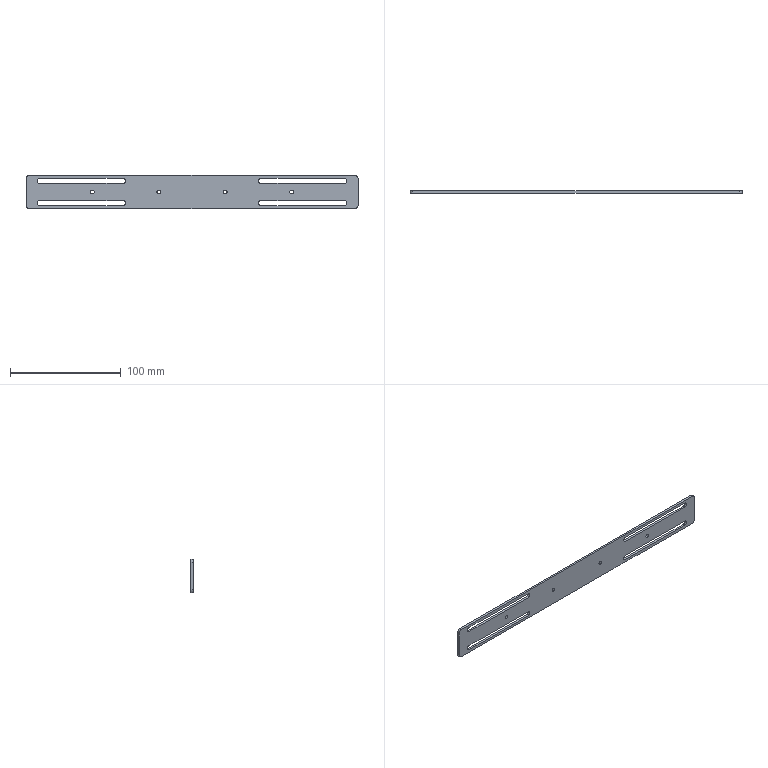Part | SolidWorks | features HoleWzd 2, Fillet 1, FlatPattern 1, SMBaseFlange 1, SheetMetal 1 | 1 solid | 34 faces | box 300 x 2 x 30 mm | volume 15076 mm3 | cylinder 20 | plane 14 | commonest cylinder face diameters 3.3 x8 4.5 x8 5 x4
STEP:
#1=CARTESIAN_POINT('',(-30.,-2.,-1.65));
#2=VERTEX_POINT('',#1);
#3=CARTESIAN_POINT('',(-30.,-2.,1.65));
#4=VERTEX_POINT('',#3);
#5=CARTESIAN_POINT('',(-30.,-2.,0.));
#6=DIRECTION('',(0.,1.,0.));
#7=DIRECTION('',(0.,0.,1.));
#8=AXIS2_PLACEMENT_3D('',#5,#6,#7);
#9=CIRCLE('',#8,1.65);
#10=EDGE_CURVE('',#2,#4,#9,.T.);
#11=ORIENTED_EDGE('',*,*,#10,.F.);
#12=CARTESIAN_POINT('',(-30.,0.,-1.65));
#13=VERTEX_POINT('',#12);
#14=CARTESIAN_POINT('',(-30.,0.,-1.65));
#15=DIRECTION('',(0.,1.,0.));
#16=VECTOR('',#15,1000.);
#17=LINE('',#14,#16);
#18=EDGE_CURVE('',#2,#13,#17,.T.);
#19=ORIENTED_EDGE('',*,*,#18,.T.);
#20=CARTESIAN_POINT('',(-30.,0.,1.65));
#21=VERTEX_POINT('',#20);
#22=CARTESIAN_POINT('',(-30.,0.,0.));
#23=DIRECTION('',(0.,1.,0.));
#24=DIRECTION('',(0.,0.,1.));
#25=AXIS2_PLACEMENT_3D('',#22,#23,#24);
#26=CIRCLE('',#25,1.65);
#27=EDGE_CURVE('',#13,#21,#26,.T.);
#28=ORIENTED_EDGE('',*,*,#27,.T.);
#29=CARTESIAN_POINT('',(-30.,0.,1.65));
#30=DIRECTION('',(0.,1.,0.));
#31=VECTOR('',#30,1000.);
#32=LINE('',#29,#31);
#33=EDGE_CURVE('',#4,#21,#32,.T.);
#34=ORIENTED_EDGE('',*,*,#33,.F.);
#35=EDGE_LOOP('',(#11,#19,#28,#34));
#36=FACE_OUTER_BOUND('',#35,.T.);
#37=CARTESIAN_POINT('',(-30.,0.,0.));
#38=DIRECTION('',(0.,1.,0.));
#39=DIRECTION('',(0.,0.,1.));
#40=AXIS2_PLACEMENT_3D('',#37,#38,#39);
#41=CYLINDRICAL_SURFACE('',#40,1.65);
#42=ADVANCED_FACE('',(#36),#41,.F.);
#43=CARTESIAN_POINT('',(30.,-2.,-1.65));
#44=VERTEX_POINT('',#43);
#45=CARTESIAN_POINT('',(30.,-2.,1.65));
#46=VERTEX_POINT('',#45);
#47=CARTESIAN_POINT('',(30.,-2.,0.));
#48=DIRECTION('',(0.,1.,0.));
#49=DIRECTION('',(0.,0.,1.));
#50=AXIS2_PLACEMENT_3D('',#47,#48,#49);
#51=CIRCLE('',#50,1.65);
#52=EDGE_CURVE('',#44,#46,#51,.T.);
#53=ORIENTED_EDGE('',*,*,#52,.F.);
#54=CARTESIAN_POINT('',(30.,0.,-1.65));
#55=VERTEX_POINT('',#54);
#56=CARTESIAN_POINT('',(30.,0.,-1.65));
#57=DIRECTION('',(0.,1.,0.));
#58=VECTOR('',#57,1000.);
#59=LINE('',#56,#58);
#60=EDGE_CURVE('',#44,#55,#59,.T.);
#61=ORIENTED_EDGE('',*,*,#60,.T.);
#62=CARTESIAN_POINT('',(30.,0.,1.65));
#63=VERTEX_POINT('',#62);
#64=CARTESIAN_POINT('',(30.,0.,0.));
#65=DIRECTION('',(0.,1.,0.));
#66=DIRECTION('',(0.,0.,1.));
#67=AXIS2_PLACEMENT_3D('',#64,#65,#66);
#68=CIRCLE('',#67,1.65);
#69=EDGE_CURVE('',#55,#63,#68,.T.);
#70=ORIENTED_EDGE('',*,*,#69,.T.);
#71=CARTESIAN_POINT('',(30.,0.,1.65));
#72=DIRECTION('',(0.,1.,0.));
#73=VECTOR('',#72,1000.);
#74=LINE('',#71,#73);
#75=EDGE_CURVE('',#46,#63,#74,.T.);
#76=ORIENTED_EDGE('',*,*,#75,.F.);
#77=EDGE_LOOP('',(#53,#61,#70,#76));
#78=FACE_OUTER_BOUND('',#77,.T.);
#79=CARTESIAN_POINT('',(30.,0.,0.));
#80=DIRECTION('',(0.,1.,0.));
#81=DIRECTION('',(0.,0.,1.));
#82=AXIS2_PLACEMENT_3D('',#79,#80,#81);
#83=CYLINDRICAL_SURFACE('',#82,1.65);
#84=ADVANCED_FACE('',(#78),#83,.F.);
#85=CARTESIAN_POINT('',(-90.,-2.,-1.65));
#86=VERTEX_POINT('',#85);
#87=CARTESIAN_POINT('',(-90.,-2.,1.65));
#88=VERTEX_POINT('',#87);
#89=CARTESIAN_POINT('',(-90.,-2.,0.));
#90=DIRECTION('',(0.,1.,0.));
#91=DIRECTION('',(0.,0.,1.));
#92=AXIS2_PLACEMENT_3D('',#89,#90,#91);
#93=CIRCLE('',#92,1.65);
#94=EDGE_CURVE('',#86,#88,#93,.T.);
#95=ORIENTED_EDGE('',*,*,#94,.F.);
#96=CARTESIAN_POINT('',(-90.,0.,-1.65));
#97=VERTEX_POINT('',#96);
#98=CARTESIAN_POINT('',(-90.,0.,-1.65));
#99=DIRECTION('',(0.,1.,0.));
#100=VECTOR('',#99,1000.);
#101=LINE('',#98,#100);
#102=EDGE_CURVE('',#86,#97,#101,.T.);
#103=ORIENTED_EDGE('',*,*,#102,.T.);
#104=CARTESIAN_POINT('',(-90.,0.,1.65));
#105=VERTEX_POINT('',#104);
#106=CARTESIAN_POINT('',(-90.,0.,0.));
#107=DIRECTION('',(0.,1.,0.));
#108=DIRECTION('',(0.,0.,1.));
#109=AXIS2_PLACEMENT_3D('',#106,#107,#108);
#110=CIRCLE('',#109,1.65);
#111=EDGE_CURVE('',#97,#105,#110,.T.);
#112=ORIENTED_EDGE('',*,*,#111,.T.);
#113=CARTESIAN_POINT('',(-90.,0.,1.65));
#114=DIRECTION('',(0.,1.,0.));
#115=VECTOR('',#114,1000.);
#116=LINE('',#113,#115);
#117=EDGE_CURVE('',#88,#105,#116,.T.);
#118=ORIENTED_EDGE('',*,*,#117,.F.);
#119=EDGE_LOOP('',(#95,#103,#112,#118));
#120=FACE_OUTER_BOUND('',#119,.T.);
#121=CARTESIAN_POINT('',(-90.,0.,0.));
#122=DIRECTION('',(0.,1.,0.));
#123=DIRECTION('',(0.,0.,1.));
#124=AXIS2_PLACEMENT_3D('',#121,#122,#123);
#125=CYLINDRICAL_SURFACE('',#124,1.65);
#126=ADVANCED_FACE('',(#120),#125,.F.);
#127=CARTESIAN_POINT('',(90.,-2.,-1.65));
#128=VERTEX_POINT('',#127);
#129=CARTESIAN_POINT('',(90.,-2.,1.65));
#130=VERTEX_POINT('',#129);
#131=CARTESIAN_POINT('',(90.,-2.,0.));
#132=DIRECTION('',(0.,1.,0.));
#133=DIRECTION('',(0.,0.,1.));
#134=AXIS2_PLACEMENT_3D('',#131,#132,#133);
#135=CIRCLE('',#134,1.65);
#136=EDGE_CURVE('',#128,#130,#135,.T.);
#137=ORIENTED_EDGE('',*,*,#136,.F.);
#138=CARTESIAN_POINT('',(90.,0.,-1.65));
#139=VERTEX_POINT('',#138);
#140=CARTESIAN_POINT('',(90.,0.,-1.65));
#141=DIRECTION('',(0.,1.,0.));
#142=VECTOR('',#141,1000.);
#143=LINE('',#140,#142);
#144=EDGE_CURVE('',#128,#139,#143,.T.);
#145=ORIENTED_EDGE('',*,*,#144,.T.);
#146=CARTESIAN_POINT('',(90.,0.,1.65));
#147=VERTEX_POINT('',#146);
#148=CARTESIAN_POINT('',(90.,0.,0.));
#149=DIRECTION('',(0.,1.,0.));
#150=DIRECTION('',(0.,0.,1.));
#151=AXIS2_PLACEMENT_3D('',#148,#149,#150);
#152=CIRCLE('',#151,1.65);
#153=EDGE_CURVE('',#139,#147,#152,.T.);
#154=ORIENTED_EDGE('',*,*,#153,.T.);
#155=CARTESIAN_POINT('',(90.,0.,1.65));
#156=DIRECTION('',(0.,1.,0.));
#157=VECTOR('',#156,1000.);
#158=LINE('',#155,#157);
#159=EDGE_CURVE('',#130,#147,#158,.T.);
#160=ORIENTED_EDGE('',*,*,#159,.F.);
#161=EDGE_LOOP('',(#137,#145,#154,#160));
#162=FACE_OUTER_BOUND('',#161,.T.);
#163=CARTESIAN_POINT('',(90.,0.,0.));
#164=DIRECTION('',(0.,1.,0.));
#165=DIRECTION('',(0.,0.,1.));
#166=AXIS2_PLACEMENT_3D('',#163,#164,#165);
#167=CYLINDRICAL_SURFACE('',#166,1.65);
#168=ADVANCED_FACE('',(#162),#167,.F.);
#169=CARTESIAN_POINT('',(147.5,-2.,-15.));
#170=VERTEX_POINT('',#169);
#171=CARTESIAN_POINT('',(-147.5,-2.,-15.));
#172=VERTEX_POINT('',#171);
#173=CARTESIAN_POINT('',(-150.,-2.,-15.));
#174=DIRECTION('',(-1.,0.,0.));
#175=VECTOR('',#174,1000.);
#176=LINE('',#173,#175);
#177=EDGE_CURVE('',#170,#172,#176,.T.);
#178=ORIENTED_EDGE('',*,*,#177,.F.);
#179=CARTESIAN_POINT('',(150.,-2.,-12.5));
#180=VERTEX_POINT('',#179);
#181=CARTESIAN_POINT('',(147.5,-2.,-12.5));
#182=DIRECTION('',(0.,-1.,0.));
#183=DIRECTION('',(0.,0.,1.));
#184=AXIS2_PLACEMENT_3D('',#181,#182,#183);
#185=CIRCLE('',#184,2.5);
#186=EDGE_CURVE('',#170,#180,#185,.T.);
#187=ORIENTED_EDGE('',*,*,#186,.T.);
#188=CARTESIAN_POINT('',(150.,-2.,12.5));
#189=VERTEX_POINT('',#188);
#190=CARTESIAN_POINT('',(150.,-2.,-15.));
#191=DIRECTION('',(0.,0.,-1.));
#192=VECTOR('',#191,1000.);
#193=LINE('',#190,#192);
#194=EDGE_CURVE('',#189,#180,#193,.T.);
#195=ORIENTED_EDGE('',*,*,#194,.F.);
#196=CARTESIAN_POINT('',(147.5,-2.,15.));
#197=VERTEX_POINT('',#196);
#198=CARTESIAN_POINT('',(147.5,-2.,12.5));
#199=DIRECTION('',(0.,-1.,0.));
#200=DIRECTION('',(0.,0.,1.));
#201=AXIS2_PLACEMENT_3D('',#198,#199,#200);
#202=CIRCLE('',#201,2.5);
#203=EDGE_CURVE('',#189,#197,#202,.T.);
#204=ORIENTED_EDGE('',*,*,#203,.T.);
#205=CARTESIAN_POINT('',(-147.5,-2.,15.));
#206=VERTEX_POINT('',#205);
#207=CARTESIAN_POINT('',(-150.,-2.,15.));
#208=DIRECTION('',(1.,0.,0.));
#209=VECTOR('',#208,1000.);
#210=LINE('',#207,#209);
#211=EDGE_CURVE('',#206,#197,#210,.T.);
#212=ORIENTED_EDGE('',*,*,#211,.F.);
#213=CARTESIAN_POINT('',(-150.,-2.,12.5));
#214=VERTEX_POINT('',#213);
#215=CARTESIAN_POINT('',(-147.5,-2.,12.5));
#216=DIRECTION('',(0.,-1.,0.));
#217=DIRECTION('',(0.,0.,1.));
#218=AXIS2_PLACEMENT_3D('',#215,#216,#217);
#219=CIRCLE('',#218,2.5);
#220=EDGE_CURVE('',#206,#214,#219,.T.);
#221=ORIENTED_EDGE('',*,*,#220,.T.);
#222=CARTESIAN_POINT('',(-150.,-2.,-12.5));
#223=VERTEX_POINT('',#222);
#224=CARTESIAN_POINT('',(-150.,-2.,-15.));
#225=DIRECTION('',(0.,0.,1.));
#226=VECTOR('',#225,1000.);
#227=LINE('',#224,#226);
#228=EDGE_CURVE('',#223,#214,#227,.T.);
#229=ORIENTED_EDGE('',*,*,#228,.F.);
#230=CARTESIAN_POINT('',(-147.5,-2.,-12.5));
#231=DIRECTION('',(0.,-1.,0.));
#232=DIRECTION('',(0.,0.,1.));
#233=AXIS2_PLACEMENT_3D('',#230,#231,#232);
#234=CIRCLE('',#233,2.5);
#235=EDGE_CURVE('',#223,#172,#234,.T.);
#236=ORIENTED_EDGE('',*,*,#235,.T.);
#237=EDGE_LOOP('',(#178,#187,#195,#204,#212,#221,#229,#236));
#238=FACE_OUTER_BOUND('',#237,.T.);
#239=CARTESIAN_POINT('',(90.,-2.,0.));
#240=DIRECTION('',(0.,1.,0.));
#241=DIRECTION('',(0.,0.,1.));
#242=AXIS2_PLACEMENT_3D('',#239,#240,#241);
#243=CIRCLE('',#242,1.65);
#244=EDGE_CURVE('',#130,#128,#243,.T.);
#245=ORIENTED_EDGE('',*,*,#244,.T.);
#246=ORIENTED_EDGE('',*,*,#136,.T.);
#247=EDGE_LOOP('',(#245,#246));
#248=FACE_BOUND('',#247,.T.);
#249=CARTESIAN_POINT('',(-90.,-2.,0.));
#250=DIRECTION('',(0.,1.,0.));
#251=DIRECTION('',(0.,0.,1.));
#252=AXIS2_PLACEMENT_3D('',#249,#250,#251);
#253=CIRCLE('',#252,1.65);
#254=EDGE_CURVE('',#88,#86,#253,.T.);
#255=ORIENTED_EDGE('',*,*,#254,.T.);
#256=ORIENTED_EDGE('',*,*,#94,.T.);
#257=EDGE_LOOP('',(#255,#256));
#258=FACE_BOUND('',#257,.T.);
#259=CARTESIAN_POINT('',(30.,-2.,0.));
#260=DIRECTION('',(0.,1.,0.));
#261=DIRECTION('',(0.,0.,1.));
#262=AXIS2_PLACEMENT_3D('',#259,#260,#261);
#263=CIRCLE('',#262,1.65);
#264=EDGE_CURVE('',#46,#44,#263,.T.);
#265=ORIENTED_EDGE('',*,*,#264,.T.);
#266=ORIENTED_EDGE('',*,*,#52,.T.);
#267=EDGE_LOOP('',(#265,#266));
#268=FACE_BOUND('',#267,.T.);
#269=CARTESIAN_POINT('',(-30.,-2.,0.));
#270=DIRECTION('',(0.,1.,0.));
#271=DIRECTION('',(0.,0.,1.));
#272=AXIS2_PLACEMENT_3D('',#269,#270,#271);
#273=CIRCLE('',#272,1.65);
#274=EDGE_CURVE('',#4,#2,#273,.T.);
#275=ORIENTED_EDGE('',*,*,#274,.T.);
#276=ORIENTED_EDGE('',*,*,#10,.T.);
#277=EDGE_LOOP('',(#275,#276));
#278=FACE_BOUND('',#277,.T.);
#279=CARTESIAN_POINT('',(-62.25,-2.,-12.25));
#280=VERTEX_POINT('',#279);
#281=CARTESIAN_POINT('',(-62.25,-2.,-7.75));
#282=VERTEX_POINT('',#281);
#283=CARTESIAN_POINT('',(-62.25,-2.,-10.));
#284=DIRECTION('',(0.,-1.,0.));
#285=DIRECTION('',(0.,0.,-1.));
#286=AXIS2_PLACEMENT_3D('',#283,#284,#285);
#287=CIRCLE('',#286,2.25);
#288=EDGE_CURVE('',#280,#282,#287,.T.);
#289=ORIENTED_EDGE('',*,*,#288,.F.);
#290=CARTESIAN_POINT('',(-137.75,-2.,-12.25));
#291=VERTEX_POINT('',#290);
#292=CARTESIAN_POINT('',(-137.75,-2.,-12.25));
#293=DIRECTION('',(1.,0.,0.));
#294=VECTOR('',#293,1000.);
#295=LINE('',#292,#294);
#296=EDGE_CURVE('',#291,#280,#295,.T.);
#297=ORIENTED_EDGE('',*,*,#296,.F.);
#298=CARTESIAN_POINT('',(-137.75,-2.,-7.75));
#299=VERTEX_POINT('',#298);
#300=CARTESIAN_POINT('',(-137.75,-2.,-10.));
#301=DIRECTION('',(0.,-1.,0.));
#302=DIRECTION('',(0.,0.,-1.));
#303=AXIS2_PLACEMENT_3D('',#300,#301,#302);
#304=CIRCLE('',#303,2.25);
#305=EDGE_CURVE('',#299,#291,#304,.T.);
#306=ORIENTED_EDGE('',*,*,#305,.F.);
#307=CARTESIAN_POINT('',(-137.75,-2.,-7.75));
#308=DIRECTION('',(1.,0.,0.));
#309=VECTOR('',#308,1000.);
#310=LINE('',#307,#309);
#311=EDGE_CURVE('',#299,#282,#310,.T.);
#312=ORIENTED_EDGE('',*,*,#311,.T.);
#313=EDGE_LOOP('',(#289,#297,#306,#312));
#314=FACE_BOUND('',#313,.T.);
#315=CARTESIAN_POINT('',(62.25,-2.,-7.75));
#316=VERTEX_POINT('',#315);
#317=CARTESIAN_POINT('',(137.75,-2.,-7.75));
#318=VERTEX_POINT('',#317);
#319=CARTESIAN_POINT('',(62.25,-2.,-7.75));
#320=DIRECTION('',(1.,0.,0.));
#321=VECTOR('',#320,1000.);
#322=LINE('',#319,#321);
#323=EDGE_CURVE('',#316,#318,#322,.T.);
#324=ORIENTED_EDGE('',*,*,#323,.T.);
#325=CARTESIAN_POINT('',(137.75,-2.,-12.25));
#326=VERTEX_POINT('',#325);
#327=CARTESIAN_POINT('',(137.75,-2.,-10.));
#328=DIRECTION('',(0.,-1.,0.));
#329=DIRECTION('',(0.,0.,-1.));
#330=AXIS2_PLACEMENT_3D('',#327,#328,#329);
#331=CIRCLE('',#330,2.25);
#332=EDGE_CURVE('',#326,#318,#331,.T.);
#333=ORIENTED_EDGE('',*,*,#332,.F.);
#334=CARTESIAN_POINT('',(62.25,-2.,-12.25));
#335=VERTEX_POINT('',#334);
#336=CARTESIAN_POINT('',(62.25,-2.,-12.25));
#337=DIRECTION('',(1.,0.,0.));
#338=VECTOR('',#337,1000.);
#339=LINE('',#336,#338);
#340=EDGE_CURVE('',#335,#326,#339,.T.);
#341=ORIENTED_EDGE('',*,*,#340,.F.);
#342=CARTESIAN_POINT('',(62.25,-2.,-10.));
#343=DIRECTION('',(0.,-1.,0.));
#344=DIRECTION('',(0.,0.,-1.));
#345=AXIS2_PLACEMENT_3D('',#342,#343,#344);
#346=CIRCLE('',#345,2.25);
#347=EDGE_CURVE('',#316,#335,#346,.T.);
#348=ORIENTED_EDGE('',*,*,#347,.F.);
#349=EDGE_LOOP('',(#324,#333,#341,#348));
#350=FACE_BOUND('',#349,.T.);
#351=CARTESIAN_POINT('',(62.25,-2.,12.25));
#352=VERTEX_POINT('',#351);
#353=CARTESIAN_POINT('',(62.25,-2.,7.75));
#354=VERTEX_POINT('',#353);
#355=CARTESIAN_POINT('',(62.25,-2.,10.));
#356=DIRECTION('',(0.,-1.,0.));
#357=DIRECTION('',(0.,0.,-1.));
#358=AXIS2_PLACEMENT_3D('',#355,#356,#357);
#359=CIRCLE('',#358,2.25);
#360=EDGE_CURVE('',#352,#354,#359,.T.);
#361=ORIENTED_EDGE('',*,*,#360,.F.);
#362=CARTESIAN_POINT('',(137.75,-2.,12.25));
#363=VERTEX_POINT('',#362);
#364=CARTESIAN_POINT('',(62.25,-2.,12.25));
#365=DIRECTION('',(1.,0.,0.));
#366=VECTOR('',#365,1000.);
#367=LINE('',#364,#366);
#368=EDGE_CURVE('',#352,#363,#367,.T.);
#369=ORIENTED_EDGE('',*,*,#368,.T.);
#370=CARTESIAN_POINT('',(137.75,-2.,7.75));
#371=VERTEX_POINT('',#370);
#372=CARTESIAN_POINT('',(137.75,-2.,10.));
#373=DIRECTION('',(0.,-1.,0.));
#374=DIRECTION('',(0.,0.,-1.));
#375=AXIS2_PLACEMENT_3D('',#372,#373,#374);
#376=CIRCLE('',#375,2.25);
#377=EDGE_CURVE('',#371,#363,#376,.T.);
#378=ORIENTED_EDGE('',*,*,#377,.F.);
#379=CARTESIAN_POINT('',(62.25,-2.,7.75));
#380=DIRECTION('',(1.,0.,0.));
#381=VECTOR('',#380,1000.);
#382=LINE('',#379,#381);
#383=EDGE_CURVE('',#354,#371,#382,.T.);
#384=ORIENTED_EDGE('',*,*,#383,.F.);
#385=EDGE_LOOP('',(#361,#369,#378,#384));
#386=FACE_BOUND('',#385,.T.);
#387=CARTESIAN_POINT('',(-62.25,-2.,7.75));
#388=VERTEX_POINT('',#387);
#389=CARTESIAN_POINT('',(-62.25,-2.,12.25));
#390=VERTEX_POINT('',#389);
#391=CARTESIAN_POINT('',(-62.25,-2.,10.));
#392=DIRECTION('',(0.,-1.,0.));
#393=DIRECTION('',(0.,0.,-1.));
#394=AXIS2_PLACEMENT_3D('',#391,#392,#393);
#395=CIRCLE('',#394,2.25);
#396=EDGE_CURVE('',#388,#390,#395,.T.);
#397=ORIENTED_EDGE('',*,*,#396,.F.);
#398=CARTESIAN_POINT('',(-137.75,-2.,7.75));
#399=VERTEX_POINT('',#398);
#400=CARTESIAN_POINT('',(-137.75,-2.,7.75));
#401=DIRECTION('',(1.,0.,0.));
#402=VECTOR('',#401,1000.);
#403=LINE('',#400,#402);
#404=EDGE_CURVE('',#399,#388,#403,.T.);
#405=ORIENTED_EDGE('',*,*,#404,.F.);
#406=CARTESIAN_POINT('',(-137.75,-2.,12.25));
#407=VERTEX_POINT('',#406);
#408=CARTESIAN_POINT('',(-137.75,-2.,10.));
#409=DIRECTION('',(0.,-1.,0.));
#410=DIRECTION('',(0.,0.,-1.));
#411=AXIS2_PLACEMENT_3D('',#408,#409,#410);
#412=CIRCLE('',#411,2.25);
#413=EDGE_CURVE('',#407,#399,#412,.T.);
#414=ORIENTED_EDGE('',*,*,#413,.F.);
#415=CARTESIAN_POINT('',(-137.75,-2.,12.25));
#416=DIRECTION('',(1.,0.,0.));
#417=VECTOR('',#416,1000.);
#418=LINE('',#415,#417);
#419=EDGE_CURVE('',#407,#390,#418,.T.);
#420=ORIENTED_EDGE('',*,*,#419,.T.);
#421=EDGE_LOOP('',(#397,#405,#414,#420));
#422=FACE_BOUND('',#421,.T.);
#423=CARTESIAN_POINT('',(0.,-2.,0.));
#424=DIRECTION('',(0.,1.,0.));
#425=DIRECTION('',(0.,0.,1.));
#426=AXIS2_PLACEMENT_3D('',#423,#424,#425);
#427=PLANE('',#426);
#428=ADVANCED_FACE('',(#238,#248,#258,#268,#278,#314,#350,#386,#422),#427,.F.);
#429=CARTESIAN_POINT('',(-137.75,0.,12.25));
#430=VERTEX_POINT('',#429);
#431=CARTESIAN_POINT('',(-137.75,0.,7.75));
#432=VERTEX_POINT('',#431);
#433=CARTESIAN_POINT('',(-137.75,0.,10.));
#434=DIRECTION('',(0.,-1.,0.));
#435=DIRECTION('',(0.,0.,-1.));
#436=AXIS2_PLACEMENT_3D('',#433,#434,#435);
#437=CIRCLE('',#436,2.25);
#438=EDGE_CURVE('',#430,#432,#437,.T.);
#439=ORIENTED_EDGE('',*,*,#438,.T.);
#440=CARTESIAN_POINT('',(-62.25,0.,7.75));
#441=VERTEX_POINT('',#440);
#442=CARTESIAN_POINT('',(-137.75,0.,7.75));
#443=DIRECTION('',(1.,0.,0.));
#444=VECTOR('',#443,1000.);
#445=LINE('',#442,#444);
#446=EDGE_CURVE('',#432,#441,#445,.T.);
#447=ORIENTED_EDGE('',*,*,#446,.T.);
#448=CARTESIAN_POINT('',(-62.25,0.,12.25));
#449=VERTEX_POINT('',#448);
#450=CARTESIAN_POINT('',(-62.25,0.,10.));
#451=DIRECTION('',(0.,-1.,0.));
#452=DIRECTION('',(0.,0.,-1.));
#453=AXIS2_PLACEMENT_3D('',#450,#451,#452);
#454=CIRCLE('',#453,2.25);
#455=EDGE_CURVE('',#441,#449,#454,.T.);
#456=ORIENTED_EDGE('',*,*,#455,.T.);
#457=CARTESIAN_POINT('',(-137.75,0.,12.25));
#458=DIRECTION('',(1.,0.,0.));
#459=VECTOR('',#458,1000.);
#460=LINE('',#457,#459);
#461=EDGE_CURVE('',#430,#449,#460,.T.);
#462=ORIENTED_EDGE('',*,*,#461,.F.);
#463=EDGE_LOOP('',(#439,#447,#456,#462));
#464=FACE_BOUND('',#463,.T.);
#465=CARTESIAN_POINT('',(62.25,0.,7.75));
#466=VERTEX_POINT('',#465);
#467=CARTESIAN_POINT('',(137.75,0.,7.75));
#468=VERTEX_POINT('',#467);
#469=CARTESIAN_POINT('',(62.25,0.,7.75));
#470=DIRECTION('',(1.,0.,0.));
#471=VECTOR('',#470,1000.);
#472=LINE('',#469,#471);
#473=EDGE_CURVE('',#466,#468,#472,.T.);
#474=ORIENTED_EDGE('',*,*,#473,.T.);
#475=CARTESIAN_POINT('',(137.75,0.,12.25));
#476=VERTEX_POINT('',#475);
#477=CARTESIAN_POINT('',(137.75,0.,10.));
#478=DIRECTION('',(0.,-1.,0.));
#479=DIRECTION('',(0.,0.,-1.));
#480=AXIS2_PLACEMENT_3D('',#477,#478,#479);
#481=CIRCLE('',#480,2.25);
#482=EDGE_CURVE('',#468,#476,#481,.T.);
#483=ORIENTED_EDGE('',*,*,#482,.T.);
#484=CARTESIAN_POINT('',(62.25,0.,12.25));
#485=VERTEX_POINT('',#484);
#486=CARTESIAN_POINT('',(62.25,0.,12.25));
#487=DIRECTION('',(1.,0.,0.));
#488=VECTOR('',#487,1000.);
#489=LINE('',#486,#488);
#490=EDGE_CURVE('',#485,#476,#489,.T.);
#491=ORIENTED_EDGE('',*,*,#490,.F.);
#492=CARTESIAN_POINT('',(62.25,0.,10.));
#493=DIRECTION('',(0.,-1.,0.));
#494=DIRECTION('',(0.,0.,-1.));
#495=AXIS2_PLACEMENT_3D('',#492,#493,#494);
#496=CIRCLE('',#495,2.25);
#497=EDGE_CURVE('',#485,#466,#496,.T.);
#498=ORIENTED_EDGE('',*,*,#497,.T.);
#499=EDGE_LOOP('',(#474,#483,#491,#498));
#500=FACE_BOUND('',#499,.T.);
#501=CARTESIAN_POINT('',(137.75,0.,-12.25));
#502=VERTEX_POINT('',#501);
#503=CARTESIAN_POINT('',(137.75,0.,-7.75));
#504=VERTEX_POINT('',#503);
#505=CARTESIAN_POINT('',(137.75,0.,-10.));
#506=DIRECTION('',(0.,-1.,0.));
#507=DIRECTION('',(0.,0.,-1.));
#508=AXIS2_PLACEMENT_3D('',#505,#506,#507);
#509=CIRCLE('',#508,2.25);
#510=EDGE_CURVE('',#502,#504,#509,.T.);
#511=ORIENTED_EDGE('',*,*,#510,.T.);
#512=CARTESIAN_POINT('',(62.25,0.,-7.75));
#513=VERTEX_POINT('',#512);
#514=CARTESIAN_POINT('',(62.25,0.,-7.75));
#515=DIRECTION('',(1.,0.,0.));
#516=VECTOR('',#515,1000.);
#517=LINE('',#514,#516);
#518=EDGE_CURVE('',#513,#504,#517,.T.);
#519=ORIENTED_EDGE('',*,*,#518,.F.);
#520=CARTESIAN_POINT('',(62.25,0.,-12.25));
#521=VERTEX_POINT('',#520);
#522=CARTESIAN_POINT('',(62.25,0.,-10.));
#523=DIRECTION('',(0.,-1.,0.));
#524=DIRECTION('',(0.,0.,-1.));
#525=AXIS2_PLACEMENT_3D('',#522,#523,#524);
#526=CIRCLE('',#525,2.25);
#527=EDGE_CURVE('',#513,#521,#526,.T.);
#528=ORIENTED_EDGE('',*,*,#527,.T.);
#529=CARTESIAN_POINT('',(62.25,0.,-12.25));
#530=DIRECTION('',(1.,0.,0.));
#531=VECTOR('',#530,1000.);
#532=LINE('',#529,#531);
#533=EDGE_CURVE('',#521,#502,#532,.T.);
#534=ORIENTED_EDGE('',*,*,#533,.T.);
#535=EDGE_LOOP('',(#511,#519,#528,#534));
#536=FACE_BOUND('',#535,.T.);
#537=CARTESIAN_POINT('',(-30.,0.,0.));
#538=DIRECTION('',(0.,1.,0.));
#539=DIRECTION('',(0.,0.,1.));
#540=AXIS2_PLACEMENT_3D('',#537,#538,#539);
#541=CIRCLE('',#540,1.65);
#542=EDGE_CURVE('',#21,#13,#541,.T.);
#543=ORIENTED_EDGE('',*,*,#542,.F.);
#544=ORIENTED_EDGE('',*,*,#27,.F.);
#545=EDGE_LOOP('',(#543,#544));
#546=FACE_BOUND('',#545,.T.);
#547=CARTESIAN_POINT('',(30.,0.,0.));
#548=DIRECTION('',(0.,1.,0.));
#549=DIRECTION('',(0.,0.,1.));
#550=AXIS2_PLACEMENT_3D('',#547,#548,#549);
#551=CIRCLE('',#550,1.65);
#552=EDGE_CURVE('',#63,#55,#551,.T.);
#553=ORIENTED_EDGE('',*,*,#552,.F.);
#554=ORIENTED_EDGE('',*,*,#69,.F.);
#555=EDGE_LOOP('',(#553,#554));
#556=FACE_BOUND('',#555,.T.);
#557=CARTESIAN_POINT('',(-90.,0.,0.));
#558=DIRECTION('',(0.,1.,0.));
#559=DIRECTION('',(0.,0.,1.));
#560=AXIS2_PLACEMENT_3D('',#557,#558,#559);
#561=CIRCLE('',#560,1.65);
#562=EDGE_CURVE('',#105,#97,#561,.T.);
#563=ORIENTED_EDGE('',*,*,#562,.F.);
#564=ORIENTED_EDGE('',*,*,#111,.F.);
#565=EDGE_LOOP('',(#563,#564));
#566=FACE_BOUND('',#565,.T.);
#567=CARTESIAN_POINT('',(90.,0.,0.));
#568=DIRECTION('',(0.,1.,0.));
#569=DIRECTION('',(0.,0.,1.));
#570=AXIS2_PLACEMENT_3D('',#567,#568,#569);
#571=CIRCLE('',#570,1.65);
#572=EDGE_CURVE('',#147,#139,#571,.T.);
#573=ORIENTED_EDGE('',*,*,#572,.F.);
#574=ORIENTED_EDGE('',*,*,#153,.F.);
#575=EDGE_LOOP('',(#573,#574));
#576=FACE_BOUND('',#575,.T.);
#577=CARTESIAN_POINT('',(150.,0.,12.5));
#578=VERTEX_POINT('',#577);
#579=CARTESIAN_POINT('',(150.,0.,-12.5));
#580=VERTEX_POINT('',#579);
#581=CARTESIAN_POINT('',(150.,0.,-15.));
#582=DIRECTION('',(0.,0.,-1.));
#583=VECTOR('',#582,1000.);
#584=LINE('',#581,#583);
#585=EDGE_CURVE('',#578,#580,#584,.T.);
#586=ORIENTED_EDGE('',*,*,#585,.T.);
#587=CARTESIAN_POINT('',(147.5,0.,-15.));
#588=VERTEX_POINT('',#587);
#589=CARTESIAN_POINT('',(147.5,0.,-12.5));
#590=DIRECTION('',(0.,1.,0.));
#591=DIRECTION('',(0.,0.,1.));
#592=AXIS2_PLACEMENT_3D('',#589,#590,#591);
#593=CIRCLE('',#592,2.5);
#594=EDGE_CURVE('',#580,#588,#593,.T.);
#595=ORIENTED_EDGE('',*,*,#594,.T.);
#596=CARTESIAN_POINT('',(-147.5,0.,-15.));
#597=VERTEX_POINT('',#596);
#598=CARTESIAN_POINT('',(-150.,0.,-15.));
#599=DIRECTION('',(-1.,0.,0.));
#600=VECTOR('',#599,1000.);
#601=LINE('',#598,#600);
#602=EDGE_CURVE('',#588,#597,#601,.T.);
#603=ORIENTED_EDGE('',*,*,#602,.T.);
#604=CARTESIAN_POINT('',(-150.,0.,-12.5));
#605=VERTEX_POINT('',#604);
#606=CARTESIAN_POINT('',(-147.5,0.,-12.5));
#607=DIRECTION('',(0.,1.,0.));
#608=DIRECTION('',(0.,0.,1.));
#609=AXIS2_PLACEMENT_3D('',#606,#607,#608);
#610=CIRCLE('',#609,2.5);
#611=EDGE_CURVE('',#597,#605,#610,.T.);
#612=ORIENTED_EDGE('',*,*,#611,.T.);
#613=CARTESIAN_POINT('',(-150.,0.,12.5));
#614=VERTEX_POINT('',#613);
#615=CARTESIAN_POINT('',(-150.,0.,-15.));
#616=DIRECTION('',(0.,0.,1.));
#617=VECTOR('',#616,1000.);
#618=LINE('',#615,#617);
#619=EDGE_CURVE('',#605,#614,#618,.T.);
#620=ORIENTED_EDGE('',*,*,#619,.T.);
#621=CARTESIAN_POINT('',(-147.5,0.,15.));
#622=VERTEX_POINT('',#621);
#623=CARTESIAN_POINT('',(-147.5,0.,12.5));
#624=DIRECTION('',(0.,1.,0.));
#625=DIRECTION('',(0.,0.,1.));
#626=AXIS2_PLACEMENT_3D('',#623,#624,#625);
#627=CIRCLE('',#626,2.5);
#628=EDGE_CURVE('',#614,#622,#627,.T.);
#629=ORIENTED_EDGE('',*,*,#628,.T.);
#630=CARTESIAN_POINT('',(147.5,0.,15.));
#631=VERTEX_POINT('',#630);
#632=CARTESIAN_POINT('',(-150.,0.,15.));
#633=DIRECTION('',(1.,0.,0.));
#634=VECTOR('',#633,1000.);
#635=LINE('',#632,#634);
#636=EDGE_CURVE('',#622,#631,#635,.T.);
#637=ORIENTED_EDGE('',*,*,#636,.T.);
#638=CARTESIAN_POINT('',(147.5,0.,12.5));
#639=DIRECTION('',(0.,1.,0.));
#640=DIRECTION('',(0.,0.,1.));
#641=AXIS2_PLACEMENT_3D('',#638,#639,#640);
#642=CIRCLE('',#641,2.5);
#643=EDGE_CURVE('',#631,#578,#642,.T.);
#644=ORIENTED_EDGE('',*,*,#643,.T.);
#645=EDGE_LOOP('',(#586,#595,#603,#612,#620,#629,#637,#644));
#646=FACE_OUTER_BOUND('',#645,.T.);
#647=CARTESIAN_POINT('',(-137.75,0.,-12.25));
#648=VERTEX_POINT('',#647);
#649=CARTESIAN_POINT('',(-62.25,0.,-12.25));
#650=VERTEX_POINT('',#649);
#651=CARTESIAN_POINT('',(-137.75,0.,-12.25));
#652=DIRECTION('',(1.,0.,0.));
#653=VECTOR('',#652,1000.);
#654=LINE('',#651,#653);
#655=EDGE_CURVE('',#648,#650,#654,.T.);
#656=ORIENTED_EDGE('',*,*,#655,.T.);
#657=CARTESIAN_POINT('',(-62.25,0.,-7.75));
#658=VERTEX_POINT('',#657);
#659=CARTESIAN_POINT('',(-62.25,0.,-10.));
#660=DIRECTION('',(0.,-1.,0.));
#661=DIRECTION('',(0.,0.,-1.));
#662=AXIS2_PLACEMENT_3D('',#659,#660,#661);
#663=CIRCLE('',#662,2.25);
#664=EDGE_CURVE('',#650,#658,#663,.T.);
#665=ORIENTED_EDGE('',*,*,#664,.T.);
#666=CARTESIAN_POINT('',(-137.75,0.,-7.75));
#667=VERTEX_POINT('',#666);
#668=CARTESIAN_POINT('',(-137.75,0.,-7.75));
#669=DIRECTION('',(1.,0.,0.));
#670=VECTOR('',#669,1000.);
#671=LINE('',#668,#670);
#672=EDGE_CURVE('',#667,#658,#671,.T.);
#673=ORIENTED_EDGE('',*,*,#672,.F.);
#674=CARTESIAN_POINT('',(-137.75,0.,-10.));
#675=DIRECTION('',(0.,-1.,0.));
#676=DIRECTION('',(0.,0.,-1.));
#677=AXIS2_PLACEMENT_3D('',#674,#675,#676);
#678=CIRCLE('',#677,2.25);
#679=EDGE_CURVE('',#667,#648,#678,.T.);
#680=ORIENTED_EDGE('',*,*,#679,.T.);
#681=EDGE_LOOP('',(#656,#665,#673,#680));
#682=FACE_BOUND('',#681,.T.);
#683=CARTESIAN_POINT('',(0.,0.,0.));
#684=DIRECTION('',(0.,1.,0.));
#685=DIRECTION('',(0.,0.,1.));
#686=AXIS2_PLACEMENT_3D('',#683,#684,#685);
#687=PLANE('',#686);
#688=ADVANCED_FACE('',(#464,#500,#536,#546,#556,#566,#576,#646,#682),#687,.T.);
#689=ORIENTED_EDGE('',*,*,#194,.T.);
#690=CARTESIAN_POINT('',(150.,-2.,-12.5));
#691=DIRECTION('',(0.,1.,0.));
#692=VECTOR('',#691,1000.);
#693=LINE('',#690,#692);
#694=EDGE_CURVE('',#180,#580,#693,.T.);
#695=ORIENTED_EDGE('',*,*,#694,.T.);
#696=ORIENTED_EDGE('',*,*,#585,.F.);
#697=CARTESIAN_POINT('',(150.,-2.,12.5));
#698=DIRECTION('',(0.,-1.,0.));
#699=VECTOR('',#698,1000.);
#700=LINE('',#697,#699);
#701=EDGE_CURVE('',#578,#189,#700,.T.);
#702=ORIENTED_EDGE('',*,*,#701,.T.);
#703=EDGE_LOOP('',(#689,#695,#696,#702));
#704=FACE_OUTER_BOUND('',#703,.T.);
#705=CARTESIAN_POINT('',(150.,-2.,-15.));
#706=DIRECTION('',(1.,0.,0.));
#707=DIRECTION('',(0.,0.,-1.));
#708=AXIS2_PLACEMENT_3D('',#705,#706,#707);
#709=PLANE('',#708);
#710=ADVANCED_FACE('',(#704),#709,.T.);
#711=ORIENTED_EDGE('',*,*,#211,.T.);
#712=CARTESIAN_POINT('',(147.5,-2.,15.));
#713=DIRECTION('',(0.,1.,0.));
#714=VECTOR('',#713,1000.);
#715=LINE('',#712,#714);
#716=EDGE_CURVE('',#197,#631,#715,.T.);
#717=ORIENTED_EDGE('',*,*,#716,.T.);
#718=ORIENTED_EDGE('',*,*,#636,.F.);
#719=CARTESIAN_POINT('',(-147.5,-2.,15.));
#720=DIRECTION('',(0.,-1.,0.));
#721=VECTOR('',#720,1000.);
#722=LINE('',#719,#721);
#723=EDGE_CURVE('',#622,#206,#722,.T.);
#724=ORIENTED_EDGE('',*,*,#723,.T.);
#725=EDGE_LOOP('',(#711,#717,#718,#724));
#726=FACE_OUTER_BOUND('',#725,.T.);
#727=CARTESIAN_POINT('',(-150.,-2.,15.));
#728=DIRECTION('',(0.,0.,1.));
#729=DIRECTION('',(1.,0.,0.));
#730=AXIS2_PLACEMENT_3D('',#727,#728,#729);
#731=PLANE('',#730);
#732=ADVANCED_FACE('',(#726),#731,.T.);
#733=ORIENTED_EDGE('',*,*,#619,.F.);
#734=CARTESIAN_POINT('',(-150.,-2.,-12.5));
#735=DIRECTION('',(0.,-1.,0.));
#736=VECTOR('',#735,1000.);
#737=LINE('',#734,#736);
#738=EDGE_CURVE('',#605,#223,#737,.T.);
#739=ORIENTED_EDGE('',*,*,#738,.T.);
#740=ORIENTED_EDGE('',*,*,#228,.T.);
#741=CARTESIAN_POINT('',(-150.,-2.,12.5));
#742=DIRECTION('',(0.,1.,0.));
#743=VECTOR('',#742,1000.);
#744=LINE('',#741,#743);
#745=EDGE_CURVE('',#214,#614,#744,.T.);
#746=ORIENTED_EDGE('',*,*,#745,.T.);
#747=EDGE_LOOP('',(#733,#739,#740,#746));
#748=FACE_OUTER_BOUND('',#747,.T.);
#749=CARTESIAN_POINT('',(-150.,-2.,-15.));
#750=DIRECTION('',(-1.,0.,0.));
#751=DIRECTION('',(0.,0.,1.));
#752=AXIS2_PLACEMENT_3D('',#749,#750,#751);
#753=PLANE('',#752);
#754=ADVANCED_FACE('',(#748),#753,.T.);
#755=ORIENTED_EDGE('',*,*,#602,.F.);
#756=CARTESIAN_POINT('',(147.5,-2.,-15.));
#757=DIRECTION('',(0.,-1.,0.));
#758=VECTOR('',#757,1000.);
#759=LINE('',#756,#758);
#760=EDGE_CURVE('',#588,#170,#759,.T.);
#761=ORIENTED_EDGE('',*,*,#760,.T.);
#762=ORIENTED_EDGE('',*,*,#177,.T.);
#763=CARTESIAN_POINT('',(-147.5,-2.,-15.));
#764=DIRECTION('',(0.,1.,0.));
#765=VECTOR('',#764,1000.);
#766=LINE('',#763,#765);
#767=EDGE_CURVE('',#172,#597,#766,.T.);
#768=ORIENTED_EDGE('',*,*,#767,.T.);
#769=EDGE_LOOP('',(#755,#761,#762,#768));
#770=FACE_OUTER_BOUND('',#769,.T.);
#771=CARTESIAN_POINT('',(-150.,-2.,-15.));
#772=DIRECTION('',(0.,0.,-1.));
#773=DIRECTION('',(-1.,0.,0.));
#774=AXIS2_PLACEMENT_3D('',#771,#772,#773);
#775=PLANE('',#774);
#776=ADVANCED_FACE('',(#770),#775,.T.);
#777=ORIENTED_EDGE('',*,*,#144,.F.);
#778=ORIENTED_EDGE('',*,*,#244,.F.);
#779=ORIENTED_EDGE('',*,*,#159,.T.);
#780=ORIENTED_EDGE('',*,*,#572,.T.);
#781=EDGE_LOOP('',(#777,#778,#779,#780));
#782=FACE_OUTER_BOUND('',#781,.T.);
#783=CARTESIAN_POINT('',(90.,0.,0.));
#784=DIRECTION('',(0.,1.,0.));
#785=DIRECTION('',(0.,0.,1.));
#786=AXIS2_PLACEMENT_3D('',#783,#784,#785);
#787=CYLINDRICAL_SURFACE('',#786,1.65);
#788=ADVANCED_FACE('',(#782),#787,.F.);
#789=ORIENTED_EDGE('',*,*,#102,.F.);
#790=ORIENTED_EDGE('',*,*,#254,.F.);
#791=ORIENTED_EDGE('',*,*,#117,.T.);
#792=ORIENTED_EDGE('',*,*,#562,.T.);
#793=EDGE_LOOP('',(#789,#790,#791,#792));
#794=FACE_OUTER_BOUND('',#793,.T.);
#795=CARTESIAN_POINT('',(-90.,0.,0.));
#796=DIRECTION('',(0.,1.,0.));
#797=DIRECTION('',(0.,0.,1.));
#798=AXIS2_PLACEMENT_3D('',#795,#796,#797);
#799=CYLINDRICAL_SURFACE('',#798,1.65);
#800=ADVANCED_FACE('',(#794),#799,.F.);
#801=ORIENTED_EDGE('',*,*,#60,.F.);
#802=ORIENTED_EDGE('',*,*,#264,.F.);
#803=ORIENTED_EDGE('',*,*,#75,.T.);
#804=ORIENTED_EDGE('',*,*,#552,.T.);
#805=EDGE_LOOP('',(#801,#802,#803,#804));
#806=FACE_OUTER_BOUND('',#805,.T.);
#807=CARTESIAN_POINT('',(30.,0.,0.));
#808=DIRECTION('',(0.,1.,0.));
#809=DIRECTION('',(0.,0.,1.));
#810=AXIS2_PLACEMENT_3D('',#807,#808,#809);
#811=CYLINDRICAL_SURFACE('',#810,1.65);
#812=ADVANCED_FACE('',(#806),#811,.F.);
#813=ORIENTED_EDGE('',*,*,#18,.F.);
#814=ORIENTED_EDGE('',*,*,#274,.F.);
#815=ORIENTED_EDGE('',*,*,#33,.T.);
#816=ORIENTED_EDGE('',*,*,#542,.T.);
#817=EDGE_LOOP('',(#813,#814,#815,#816));
#818=FACE_OUTER_BOUND('',#817,.T.);
#819=CARTESIAN_POINT('',(-30.,0.,0.));
#820=DIRECTION('',(0.,1.,0.));
#821=DIRECTION('',(0.,0.,1.));
#822=AXIS2_PLACEMENT_3D('',#819,#820,#821);
#823=CYLINDRICAL_SURFACE('',#822,1.65);
#824=ADVANCED_FACE('',(#818),#823,.F.);
#825=ORIENTED_EDGE('',*,*,#664,.F.);
#826=CARTESIAN_POINT('',(-62.25,-2.,-12.25));
#827=DIRECTION('',(0.,1.,0.));
#828=VECTOR('',#827,1000.);
#829=LINE('',#826,#828);
#830=EDGE_CURVE('',#280,#650,#829,.T.);
#831=ORIENTED_EDGE('',*,*,#830,.F.);
#832=ORIENTED_EDGE('',*,*,#288,.T.);
#833=CARTESIAN_POINT('',(-62.25,-2.,-7.75));
#834=DIRECTION('',(0.,-1.,0.));
#835=VECTOR('',#834,1000.);
#836=LINE('',#833,#835);
#837=EDGE_CURVE('',#658,#282,#836,.T.);
#838=ORIENTED_EDGE('',*,*,#837,.F.);
#839=EDGE_LOOP('',(#825,#831,#832,#838));
#840=FACE_OUTER_BOUND('',#839,.T.);
#841=CARTESIAN_POINT('',(-62.25,-2.,-10.));
#842=DIRECTION('',(0.,-1.,0.));
#843=DIRECTION('',(0.,0.,-1.));
#844=AXIS2_PLACEMENT_3D('',#841,#842,#843);
#845=CYLINDRICAL_SURFACE('',#844,2.25);
#846=ADVANCED_FACE('',(#840),#845,.F.);
#847=ORIENTED_EDGE('',*,*,#305,.T.);
#848=CARTESIAN_POINT('',(-137.75,-2.,-12.25));
#849=DIRECTION('',(0.,-1.,0.));
#850=VECTOR('',#849,1000.);
#851=LINE('',#848,#850);
#852=EDGE_CURVE('',#648,#291,#851,.T.);
#853=ORIENTED_EDGE('',*,*,#852,.F.);
#854=ORIENTED_EDGE('',*,*,#679,.F.);
#855=CARTESIAN_POINT('',(-137.75,-2.,-7.75));
#856=DIRECTION('',(0.,1.,0.));
#857=VECTOR('',#856,1000.);
#858=LINE('',#855,#857);
#859=EDGE_CURVE('',#299,#667,#858,.T.);
#860=ORIENTED_EDGE('',*,*,#859,.F.);
#861=EDGE_LOOP('',(#847,#853,#854,#860));
#862=FACE_OUTER_BOUND('',#861,.T.);
#863=CARTESIAN_POINT('',(-137.75,-2.,-10.));
#864=DIRECTION('',(0.,-1.,0.));
#865=DIRECTION('',(0.,0.,-1.));
#866=AXIS2_PLACEMENT_3D('',#863,#864,#865);
#867=CYLINDRICAL_SURFACE('',#866,2.25);
#868=ADVANCED_FACE('',(#862),#867,.F.);
#869=ORIENTED_EDGE('',*,*,#837,.T.);
#870=ORIENTED_EDGE('',*,*,#311,.F.);
#871=ORIENTED_EDGE('',*,*,#859,.T.);
#872=ORIENTED_EDGE('',*,*,#672,.T.);
#873=EDGE_LOOP('',(#869,#870,#871,#872));
#874=FACE_OUTER_BOUND('',#873,.T.);
#875=CARTESIAN_POINT('',(-137.75,-2.,-7.75));
#876=DIRECTION('',(0.,0.,1.));
#877=DIRECTION('',(1.,0.,0.));
#878=AXIS2_PLACEMENT_3D('',#875,#876,#877);
#879=PLANE('',#878);
#880=ADVANCED_FACE('',(#874),#879,.F.);
#881=ORIENTED_EDGE('',*,*,#830,.T.);
#882=ORIENTED_EDGE('',*,*,#655,.F.);
#883=ORIENTED_EDGE('',*,*,#852,.T.);
#884=ORIENTED_EDGE('',*,*,#296,.T.);
#885=EDGE_LOOP('',(#881,#882,#883,#884));
#886=FACE_OUTER_BOUND('',#885,.T.);
#887=CARTESIAN_POINT('',(-137.75,-2.,-12.25));
#888=DIRECTION('',(0.,0.,-1.));
#889=DIRECTION('',(-1.,0.,0.));
#890=AXIS2_PLACEMENT_3D('',#887,#888,#889);
#891=PLANE('',#890);
#892=ADVANCED_FACE('',(#886),#891,.F.);
#893=ORIENTED_EDGE('',*,*,#510,.F.);
#894=CARTESIAN_POINT('',(137.75,-2.,-12.25));
#895=DIRECTION('',(0.,1.,0.));
#896=VECTOR('',#895,1000.);
#897=LINE('',#894,#896);
#898=EDGE_CURVE('',#326,#502,#897,.T.);
#899=ORIENTED_EDGE('',*,*,#898,.F.);
#900=ORIENTED_EDGE('',*,*,#332,.T.);
#901=CARTESIAN_POINT('',(137.75,-2.,-7.75));
#902=DIRECTION('',(0.,-1.,0.));
#903=VECTOR('',#902,1000.);
#904=LINE('',#901,#903);
#905=EDGE_CURVE('',#504,#318,#904,.T.);
#906=ORIENTED_EDGE('',*,*,#905,.F.);
#907=EDGE_LOOP('',(#893,#899,#900,#906));
#908=FACE_OUTER_BOUND('',#907,.T.);
#909=CARTESIAN_POINT('',(137.75,-2.,-10.));
#910=DIRECTION('',(0.,-1.,0.));
#911=DIRECTION('',(0.,0.,-1.));
#912=AXIS2_PLACEMENT_3D('',#909,#910,#911);
#913=CYLINDRICAL_SURFACE('',#912,2.25);
#914=ADVANCED_FACE('',(#908),#913,.F.);
#915=ORIENTED_EDGE('',*,*,#347,.T.);
#916=CARTESIAN_POINT('',(62.25,-2.,-12.25));
#917=DIRECTION('',(0.,-1.,0.));
#918=VECTOR('',#917,1000.);
#919=LINE('',#916,#918);
#920=EDGE_CURVE('',#521,#335,#919,.T.);
#921=ORIENTED_EDGE('',*,*,#920,.F.);
#922=ORIENTED_EDGE('',*,*,#527,.F.);
#923=CARTESIAN_POINT('',(62.25,-2.,-7.75));
#924=DIRECTION('',(0.,1.,0.));
#925=VECTOR('',#924,1000.);
#926=LINE('',#923,#925);
#927=EDGE_CURVE('',#316,#513,#926,.T.);
#928=ORIENTED_EDGE('',*,*,#927,.F.);
#929=EDGE_LOOP('',(#915,#921,#922,#928));
#930=FACE_OUTER_BOUND('',#929,.T.);
#931=CARTESIAN_POINT('',(62.25,-2.,-10.));
#932=DIRECTION('',(0.,-1.,0.));
#933=DIRECTION('',(0.,0.,-1.));
#934=AXIS2_PLACEMENT_3D('',#931,#932,#933);
#935=CYLINDRICAL_SURFACE('',#934,2.25);
#936=ADVANCED_FACE('',(#930),#935,.F.);
#937=ORIENTED_EDGE('',*,*,#905,.T.);
#938=ORIENTED_EDGE('',*,*,#323,.F.);
#939=ORIENTED_EDGE('',*,*,#927,.T.);
#940=ORIENTED_EDGE('',*,*,#518,.T.);
#941=EDGE_LOOP('',(#937,#938,#939,#940));
#942=FACE_OUTER_BOUND('',#941,.T.);
#943=CARTESIAN_POINT('',(62.25,-2.,-7.75));
#944=DIRECTION('',(0.,0.,1.));
#945=DIRECTION('',(1.,0.,0.));
#946=AXIS2_PLACEMENT_3D('',#943,#944,#945);
#947=PLANE('',#946);
#948=ADVANCED_FACE('',(#942),#947,.F.);
#949=ORIENTED_EDGE('',*,*,#898,.T.);
#950=ORIENTED_EDGE('',*,*,#533,.F.);
#951=ORIENTED_EDGE('',*,*,#920,.T.);
#952=ORIENTED_EDGE('',*,*,#340,.T.);
#953=EDGE_LOOP('',(#949,#950,#951,#952));
#954=FACE_OUTER_BOUND('',#953,.T.);
#955=CARTESIAN_POINT('',(62.25,-2.,-12.25));
#956=DIRECTION('',(0.,0.,-1.));
#957=DIRECTION('',(-1.,0.,0.));
#958=AXIS2_PLACEMENT_3D('',#955,#956,#957);
#959=PLANE('',#958);
#960=ADVANCED_FACE('',(#954),#959,.F.);
#961=ORIENTED_EDGE('',*,*,#482,.F.);
#962=CARTESIAN_POINT('',(137.75,-2.,7.75));
#963=DIRECTION('',(0.,1.,0.));
#964=VECTOR('',#963,1000.);
#965=LINE('',#962,#964);
#966=EDGE_CURVE('',#371,#468,#965,.T.);
#967=ORIENTED_EDGE('',*,*,#966,.F.);
#968=ORIENTED_EDGE('',*,*,#377,.T.);
#969=CARTESIAN_POINT('',(137.75,-2.,12.25));
#970=DIRECTION('',(0.,-1.,0.));
#971=VECTOR('',#970,1000.);
#972=LINE('',#969,#971);
#973=EDGE_CURVE('',#476,#363,#972,.T.);
#974=ORIENTED_EDGE('',*,*,#973,.F.);
#975=EDGE_LOOP('',(#961,#967,#968,#974));
#976=FACE_OUTER_BOUND('',#975,.T.);
#977=CARTESIAN_POINT('',(137.75,-2.,10.));
#978=DIRECTION('',(0.,-1.,0.));
#979=DIRECTION('',(0.,0.,-1.));
#980=AXIS2_PLACEMENT_3D('',#977,#978,#979);
#981=CYLINDRICAL_SURFACE('',#980,2.25);
#982=ADVANCED_FACE('',(#976),#981,.F.);
#983=ORIENTED_EDGE('',*,*,#360,.T.);
#984=CARTESIAN_POINT('',(62.25,-2.,7.75));
#985=DIRECTION('',(0.,-1.,0.));
#986=VECTOR('',#985,1000.);
#987=LINE('',#984,#986);
#988=EDGE_CURVE('',#466,#354,#987,.T.);
#989=ORIENTED_EDGE('',*,*,#988,.F.);
#990=ORIENTED_EDGE('',*,*,#497,.F.);
#991=CARTESIAN_POINT('',(62.25,-2.,12.25));
#992=DIRECTION('',(0.,1.,0.));
#993=VECTOR('',#992,1000.);
#994=LINE('',#991,#993);
#995=EDGE_CURVE('',#352,#485,#994,.T.);
#996=ORIENTED_EDGE('',*,*,#995,.F.);
#997=EDGE_LOOP('',(#983,#989,#990,#996));
#998=FACE_OUTER_BOUND('',#997,.T.);
#999=CARTESIAN_POINT('',(62.25,-2.,10.));
#1000=DIRECTION('',(0.,-1.,0.));
#1001=DIRECTION('',(0.,0.,-1.));
#1002=AXIS2_PLACEMENT_3D('',#999,#1000,#1001);
#1003=CYLINDRICAL_SURFACE('',#1002,2.25);
#1004=ADVANCED_FACE('',(#998),#1003,.F.);
#1005=ORIENTED_EDGE('',*,*,#973,.T.);
#1006=ORIENTED_EDGE('',*,*,#368,.F.);
#1007=ORIENTED_EDGE('',*,*,#995,.T.);
#1008=ORIENTED_EDGE('',*,*,#490,.T.);
#1009=EDGE_LOOP('',(#1005,#1006,#1007,#1008));
#1010=FACE_OUTER_BOUND('',#1009,.T.);
#1011=CARTESIAN_POINT('',(62.25,-2.,12.25));
#1012=DIRECTION('',(0.,0.,1.));
#1013=DIRECTION('',(1.,0.,0.));
#1014=AXIS2_PLACEMENT_3D('',#1011,#1012,#1013);
#1015=PLANE('',#1014);
#1016=ADVANCED_FACE('',(#1010),#1015,.F.);
#1017=ORIENTED_EDGE('',*,*,#966,.T.);
#1018=ORIENTED_EDGE('',*,*,#473,.F.);
#1019=ORIENTED_EDGE('',*,*,#988,.T.);
#1020=ORIENTED_EDGE('',*,*,#383,.T.);
#1021=EDGE_LOOP('',(#1017,#1018,#1019,#1020));
#1022=FACE_OUTER_BOUND('',#1021,.T.);
#1023=CARTESIAN_POINT('',(62.25,-2.,7.75));
#1024=DIRECTION('',(0.,0.,-1.));
#1025=DIRECTION('',(-1.,0.,0.));
#1026=AXIS2_PLACEMENT_3D('',#1023,#1024,#1025);
#1027=PLANE('',#1026);
#1028=ADVANCED_FACE('',(#1022),#1027,.F.);
#1029=ORIENTED_EDGE('',*,*,#455,.F.);
#1030=CARTESIAN_POINT('',(-62.25,-2.,7.75));
#1031=DIRECTION('',(0.,1.,0.));
#1032=VECTOR('',#1031,1000.);
#1033=LINE('',#1030,#1032);
#1034=EDGE_CURVE('',#388,#441,#1033,.T.);
#1035=ORIENTED_EDGE('',*,*,#1034,.F.);
#1036=ORIENTED_EDGE('',*,*,#396,.T.);
#1037=CARTESIAN_POINT('',(-62.25,-2.,12.25));
#1038=DIRECTION('',(0.,-1.,0.));
#1039=VECTOR('',#1038,1000.);
#1040=LINE('',#1037,#1039);
#1041=EDGE_CURVE('',#449,#390,#1040,.T.);
#1042=ORIENTED_EDGE('',*,*,#1041,.F.);
#1043=EDGE_LOOP('',(#1029,#1035,#1036,#1042));
#1044=FACE_OUTER_BOUND('',#1043,.T.);
#1045=CARTESIAN_POINT('',(-62.25,-2.,10.));
#1046=DIRECTION('',(0.,-1.,0.));
#1047=DIRECTION('',(0.,0.,-1.));
#1048=AXIS2_PLACEMENT_3D('',#1045,#1046,#1047);
#1049=CYLINDRICAL_SURFACE('',#1048,2.25);
#1050=ADVANCED_FACE('',(#1044),#1049,.F.);
#1051=ORIENTED_EDGE('',*,*,#413,.T.);
#1052=CARTESIAN_POINT('',(-137.75,-2.,7.75));
#1053=DIRECTION('',(0.,-1.,0.));
#1054=VECTOR('',#1053,1000.);
#1055=LINE('',#1052,#1054);
#1056=EDGE_CURVE('',#432,#399,#1055,.T.);
#1057=ORIENTED_EDGE('',*,*,#1056,.F.);
#1058=ORIENTED_EDGE('',*,*,#438,.F.);
#1059=CARTESIAN_POINT('',(-137.75,-2.,12.25));
#1060=DIRECTION('',(0.,1.,0.));
#1061=VECTOR('',#1060,1000.);
#1062=LINE('',#1059,#1061);
#1063=EDGE_CURVE('',#407,#430,#1062,.T.);
#1064=ORIENTED_EDGE('',*,*,#1063,.F.);
#1065=EDGE_LOOP('',(#1051,#1057,#1058,#1064));
#1066=FACE_OUTER_BOUND('',#1065,.T.);
#1067=CARTESIAN_POINT('',(-137.75,-2.,10.));
#1068=DIRECTION('',(0.,-1.,0.));
#1069=DIRECTION('',(0.,0.,-1.));
#1070=AXIS2_PLACEMENT_3D('',#1067,#1068,#1069);
#1071=CYLINDRICAL_SURFACE('',#1070,2.25);
#1072=ADVANCED_FACE('',(#1066),#1071,.F.);
#1073=ORIENTED_EDGE('',*,*,#1041,.T.);
#1074=ORIENTED_EDGE('',*,*,#419,.F.);
#1075=ORIENTED_EDGE('',*,*,#1063,.T.);
#1076=ORIENTED_EDGE('',*,*,#461,.T.);
#1077=EDGE_LOOP('',(#1073,#1074,#1075,#1076));
#1078=FACE_OUTER_BOUND('',#1077,.T.);
#1079=CARTESIAN_POINT('',(-137.75,-2.,12.25));
#1080=DIRECTION('',(0.,0.,1.));
#1081=DIRECTION('',(1.,0.,0.));
#1082=AXIS2_PLACEMENT_3D('',#1079,#1080,#1081);
#1083=PLANE('',#1082);
#1084=ADVANCED_FACE('',(#1078),#1083,.F.);
#1085=ORIENTED_EDGE('',*,*,#1034,.T.);
#1086=ORIENTED_EDGE('',*,*,#446,.F.);
#1087=ORIENTED_EDGE('',*,*,#1056,.T.);
#1088=ORIENTED_EDGE('',*,*,#404,.T.);
#1089=EDGE_LOOP('',(#1085,#1086,#1087,#1088));
#1090=FACE_OUTER_BOUND('',#1089,.T.);
#1091=CARTESIAN_POINT('',(-137.75,-2.,7.75));
#1092=DIRECTION('',(0.,0.,-1.));
#1093=DIRECTION('',(-1.,0.,0.));
#1094=AXIS2_PLACEMENT_3D('',#1091,#1092,#1093);
#1095=PLANE('',#1094);
#1096=ADVANCED_FACE('',(#1090),#1095,.F.);
#1097=ORIENTED_EDGE('',*,*,#186,.F.);
#1098=ORIENTED_EDGE('',*,*,#760,.F.);
#1099=ORIENTED_EDGE('',*,*,#594,.F.);
#1100=ORIENTED_EDGE('',*,*,#694,.F.);
#1101=EDGE_LOOP('',(#1097,#1098,#1099,#1100));
#1102=FACE_OUTER_BOUND('',#1101,.T.);
#1103=CARTESIAN_POINT('',(147.5,-2.,-12.5));
#1104=DIRECTION('',(0.,1.,0.));
#1105=DIRECTION('',(0.,0.,1.));
#1106=AXIS2_PLACEMENT_3D('',#1103,#1104,#1105);
#1107=CYLINDRICAL_SURFACE('',#1106,2.5);
#1108=ADVANCED_FACE('',(#1102),#1107,.T.);
#1109=ORIENTED_EDGE('',*,*,#203,.F.);
#1110=ORIENTED_EDGE('',*,*,#701,.F.);
#1111=ORIENTED_EDGE('',*,*,#643,.F.);
#1112=ORIENTED_EDGE('',*,*,#716,.F.);
#1113=EDGE_LOOP('',(#1109,#1110,#1111,#1112));
#1114=FACE_OUTER_BOUND('',#1113,.T.);
#1115=CARTESIAN_POINT('',(147.5,-2.,12.5));
#1116=DIRECTION('',(0.,1.,0.));
#1117=DIRECTION('',(0.,0.,1.));
#1118=AXIS2_PLACEMENT_3D('',#1115,#1116,#1117);
#1119=CYLINDRICAL_SURFACE('',#1118,2.5);
#1120=ADVANCED_FACE('',(#1114),#1119,.T.);
#1121=ORIENTED_EDGE('',*,*,#235,.F.);
#1122=ORIENTED_EDGE('',*,*,#738,.F.);
#1123=ORIENTED_EDGE('',*,*,#611,.F.);
#1124=ORIENTED_EDGE('',*,*,#767,.F.);
#1125=EDGE_LOOP('',(#1121,#1122,#1123,#1124));
#1126=FACE_OUTER_BOUND('',#1125,.T.);
#1127=CARTESIAN_POINT('',(-147.5,-2.,-12.5));
#1128=DIRECTION('',(0.,1.,0.));
#1129=DIRECTION('',(0.,0.,1.));
#1130=AXIS2_PLACEMENT_3D('',#1127,#1128,#1129);
#1131=CYLINDRICAL_SURFACE('',#1130,2.5);
#1132=ADVANCED_FACE('',(#1126),#1131,.T.);
#1133=ORIENTED_EDGE('',*,*,#220,.F.);
#1134=ORIENTED_EDGE('',*,*,#723,.F.);
#1135=ORIENTED_EDGE('',*,*,#628,.F.);
#1136=ORIENTED_EDGE('',*,*,#745,.F.);
#1137=EDGE_LOOP('',(#1133,#1134,#1135,#1136));
#1138=FACE_OUTER_BOUND('',#1137,.T.);
#1139=CARTESIAN_POINT('',(-147.5,-2.,12.5));
#1140=DIRECTION('',(0.,1.,0.));
#1141=DIRECTION('',(0.,0.,1.));
#1142=AXIS2_PLACEMENT_3D('',#1139,#1140,#1141);
#1143=CYLINDRICAL_SURFACE('',#1142,2.5);
#1144=ADVANCED_FACE('',(#1138),#1143,.T.);
#1145=CLOSED_SHELL('',(#42,#84,#126,#168,#428,#688,#710,#732,#754,#776,#788,#800,#812,#824,#846,#868,#880,#892,#914,#936,#948,#960,#982,#1004,#1016,#1028,#1050,#1072,#1084,#1096,#1108,#1120,#1132,#1144));
#1146=MANIFOLD_SOLID_BREP('',#1145);
#1147=CARTESIAN_POINT('',(0.,0.,0.));
#1148=DIRECTION('',(0.,0.,1.));
#1149=DIRECTION('',(1.,0.,0.));
#1150=AXIS2_PLACEMENT_3D('',#1147,#1148,#1149);
#1151=(LENGTH_UNIT()NAMED_UNIT(*)SI_UNIT(.MILLI.,.METRE.));
#1152=UNCERTAINTY_MEASURE_WITH_UNIT(LENGTH_MEASURE(0.00001),#1151,'','');
#1153=(NAMED_UNIT(*)PLANE_ANGLE_UNIT()SI_UNIT($,.RADIAN.));
#1154=(NAMED_UNIT(*)SI_UNIT($,.STERADIAN.)SOLID_ANGLE_UNIT());
#1155=(GEOMETRIC_REPRESENTATION_CONTEXT(3)GLOBAL_UNCERTAINTY_ASSIGNED_CONTEXT((#1152))GLOBAL_UNIT_ASSIGNED_CONTEXT((#1151,#1153,#1154))REPRESENTATION_CONTEXT('',''));
#1156=ADVANCED_BREP_SHAPE_REPRESENTATION('',(#1146,#1150),#1155);